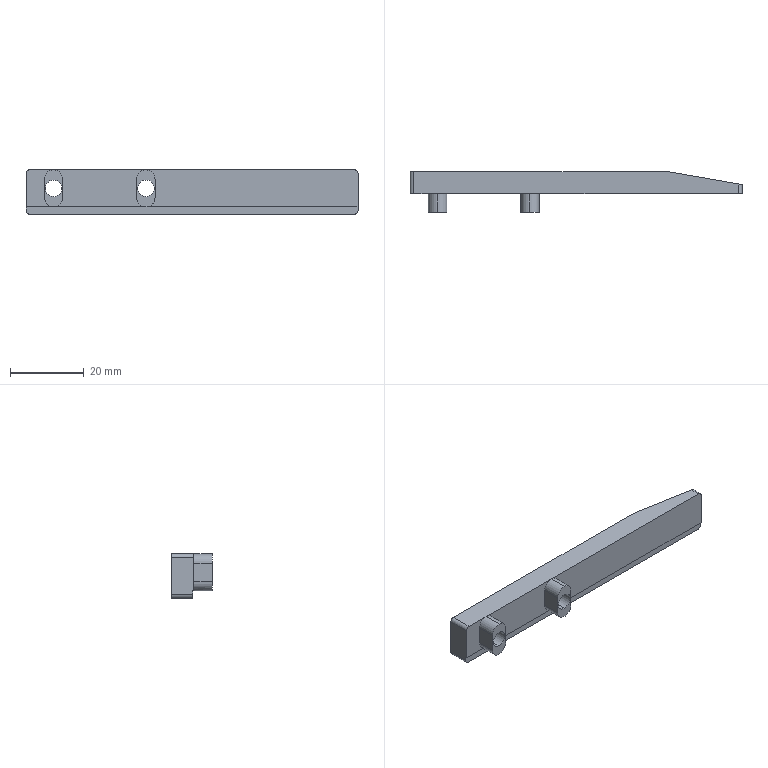Part | STEP file | 10000020606swp000-1 | 1 solid | 37 faces | box 90 x 11 x 12 mm | volume 5783 mm3 | plane 19 | cylinder 18 | commonest cylinder face diameters 5 x6 2 x4 4.5 x4 8 x4
STEP:
#1=CARTESIAN_POINT('',(7.5,1.4,-3.));
#2=VERTEX_POINT('',#1);
#3=CARTESIAN_POINT('',(7.5,1.4,5.));
#4=VERTEX_POINT('',#3);
#5=CARTESIAN_POINT('',(7.5,1.4,1.));
#6=DIRECTION('',(0.,1.,0.));
#7=DIRECTION('',(0.,0.,1.));
#8=AXIS2_PLACEMENT_3D('',#5,#6,#7);
#9=CIRCLE('',#8,4.);
#10=EDGE_CURVE('',#2,#4,#9,.T.);
#11=ORIENTED_EDGE('',*,*,#10,.F.);
#12=CARTESIAN_POINT('',(7.5,6.,-3.));
#13=VERTEX_POINT('',#12);
#14=CARTESIAN_POINT('',(7.5,6.,-3.));
#15=DIRECTION('',(0.,1.,0.));
#16=VECTOR('',#15,1000.);
#17=LINE('',#14,#16);
#18=EDGE_CURVE('',#2,#13,#17,.T.);
#19=ORIENTED_EDGE('',*,*,#18,.T.);
#20=CARTESIAN_POINT('',(7.5,6.,5.));
#21=VERTEX_POINT('',#20);
#22=CARTESIAN_POINT('',(7.5,6.,1.));
#23=DIRECTION('',(0.,1.,0.));
#24=DIRECTION('',(0.,0.,1.));
#25=AXIS2_PLACEMENT_3D('',#22,#23,#24);
#26=CIRCLE('',#25,4.);
#27=EDGE_CURVE('',#13,#21,#26,.T.);
#28=ORIENTED_EDGE('',*,*,#27,.T.);
#29=CARTESIAN_POINT('',(7.5,6.,5.));
#30=DIRECTION('',(0.,1.,0.));
#31=VECTOR('',#30,1000.);
#32=LINE('',#29,#31);
#33=EDGE_CURVE('',#4,#21,#32,.T.);
#34=ORIENTED_EDGE('',*,*,#33,.F.);
#35=EDGE_LOOP('',(#11,#19,#28,#34));
#36=FACE_OUTER_BOUND('',#35,.T.);
#37=CARTESIAN_POINT('',(7.5,6.,1.));
#38=DIRECTION('',(0.,1.,0.));
#39=DIRECTION('',(0.,0.,1.));
#40=AXIS2_PLACEMENT_3D('',#37,#38,#39);
#41=CYLINDRICAL_SURFACE('',#40,4.);
#42=ADVANCED_FACE('',(#36),#41,.F.);
#43=CARTESIAN_POINT('',(7.5,-5.,3.25));
#44=VERTEX_POINT('',#43);
#45=CARTESIAN_POINT('',(7.5,-5.,-1.25));
#46=VERTEX_POINT('',#45);
#47=CARTESIAN_POINT('',(7.5,-5.,1.));
#48=DIRECTION('',(0.,-1.,0.));
#49=DIRECTION('',(0.,0.,-1.));
#50=AXIS2_PLACEMENT_3D('',#47,#48,#49);
#51=CIRCLE('',#50,2.25);
#52=EDGE_CURVE('',#44,#46,#51,.T.);
#53=ORIENTED_EDGE('',*,*,#52,.T.);
#54=CARTESIAN_POINT('',(7.5,1.4,-1.25));
#55=VERTEX_POINT('',#54);
#56=CARTESIAN_POINT('',(7.5,6.,-1.25));
#57=DIRECTION('',(0.,1.,0.));
#58=VECTOR('',#57,1000.);
#59=LINE('',#56,#58);
#60=EDGE_CURVE('',#46,#55,#59,.T.);
#61=ORIENTED_EDGE('',*,*,#60,.T.);
#62=CARTESIAN_POINT('',(7.5,1.4,3.25));
#63=VERTEX_POINT('',#62);
#64=CARTESIAN_POINT('',(7.5,1.4,1.));
#65=DIRECTION('',(0.,1.,0.));
#66=DIRECTION('',(0.,0.,1.));
#67=AXIS2_PLACEMENT_3D('',#64,#65,#66);
#68=CIRCLE('',#67,2.25);
#69=EDGE_CURVE('',#55,#63,#68,.T.);
#70=ORIENTED_EDGE('',*,*,#69,.T.);
#71=CARTESIAN_POINT('',(7.5,6.,3.25));
#72=DIRECTION('',(0.,1.,0.));
#73=VECTOR('',#72,1000.);
#74=LINE('',#71,#73);
#75=EDGE_CURVE('',#44,#63,#74,.T.);
#76=ORIENTED_EDGE('',*,*,#75,.F.);
#77=EDGE_LOOP('',(#53,#61,#70,#76));
#78=FACE_OUTER_BOUND('',#77,.T.);
#79=CARTESIAN_POINT('',(7.5,6.,1.));
#80=DIRECTION('',(0.,1.,0.));
#81=DIRECTION('',(0.,0.,1.));
#82=AXIS2_PLACEMENT_3D('',#79,#80,#81);
#83=CYLINDRICAL_SURFACE('',#82,2.25);
#84=ADVANCED_FACE('',(#78),#83,.F.);
#85=CARTESIAN_POINT('',(32.5,1.4,-3.));
#86=VERTEX_POINT('',#85);
#87=CARTESIAN_POINT('',(32.5,1.4,5.));
#88=VERTEX_POINT('',#87);
#89=CARTESIAN_POINT('',(32.5,1.4,1.));
#90=DIRECTION('',(0.,1.,0.));
#91=DIRECTION('',(0.,0.,1.));
#92=AXIS2_PLACEMENT_3D('',#89,#90,#91);
#93=CIRCLE('',#92,4.);
#94=EDGE_CURVE('',#86,#88,#93,.T.);
#95=ORIENTED_EDGE('',*,*,#94,.F.);
#96=CARTESIAN_POINT('',(32.5,6.,-3.));
#97=VERTEX_POINT('',#96);
#98=CARTESIAN_POINT('',(32.5,6.,-3.));
#99=DIRECTION('',(0.,1.,0.));
#100=VECTOR('',#99,1000.);
#101=LINE('',#98,#100);
#102=EDGE_CURVE('',#86,#97,#101,.T.);
#103=ORIENTED_EDGE('',*,*,#102,.T.);
#104=CARTESIAN_POINT('',(32.5,6.,5.));
#105=VERTEX_POINT('',#104);
#106=CARTESIAN_POINT('',(32.5,6.,1.));
#107=DIRECTION('',(0.,1.,0.));
#108=DIRECTION('',(0.,0.,1.));
#109=AXIS2_PLACEMENT_3D('',#106,#107,#108);
#110=CIRCLE('',#109,4.);
#111=EDGE_CURVE('',#97,#105,#110,.T.);
#112=ORIENTED_EDGE('',*,*,#111,.T.);
#113=CARTESIAN_POINT('',(32.5,6.,5.));
#114=DIRECTION('',(0.,1.,0.));
#115=VECTOR('',#114,1000.);
#116=LINE('',#113,#115);
#117=EDGE_CURVE('',#88,#105,#116,.T.);
#118=ORIENTED_EDGE('',*,*,#117,.F.);
#119=EDGE_LOOP('',(#95,#103,#112,#118));
#120=FACE_OUTER_BOUND('',#119,.T.);
#121=CARTESIAN_POINT('',(32.5,6.,1.));
#122=DIRECTION('',(0.,1.,0.));
#123=DIRECTION('',(0.,0.,1.));
#124=AXIS2_PLACEMENT_3D('',#121,#122,#123);
#125=CYLINDRICAL_SURFACE('',#124,4.);
#126=ADVANCED_FACE('',(#120),#125,.F.);
#127=CARTESIAN_POINT('',(32.5,-5.,3.25));
#128=VERTEX_POINT('',#127);
#129=CARTESIAN_POINT('',(32.5,-5.,-1.25));
#130=VERTEX_POINT('',#129);
#131=CARTESIAN_POINT('',(32.5,-5.,1.));
#132=DIRECTION('',(0.,-1.,0.));
#133=DIRECTION('',(0.,0.,-1.));
#134=AXIS2_PLACEMENT_3D('',#131,#132,#133);
#135=CIRCLE('',#134,2.25);
#136=EDGE_CURVE('',#128,#130,#135,.T.);
#137=ORIENTED_EDGE('',*,*,#136,.T.);
#138=CARTESIAN_POINT('',(32.5,1.4,-1.25));
#139=VERTEX_POINT('',#138);
#140=CARTESIAN_POINT('',(32.5,6.,-1.25));
#141=DIRECTION('',(0.,1.,0.));
#142=VECTOR('',#141,1000.);
#143=LINE('',#140,#142);
#144=EDGE_CURVE('',#130,#139,#143,.T.);
#145=ORIENTED_EDGE('',*,*,#144,.T.);
#146=CARTESIAN_POINT('',(32.5,1.4,3.25));
#147=VERTEX_POINT('',#146);
#148=CARTESIAN_POINT('',(32.5,1.4,1.));
#149=DIRECTION('',(0.,1.,0.));
#150=DIRECTION('',(0.,0.,1.));
#151=AXIS2_PLACEMENT_3D('',#148,#149,#150);
#152=CIRCLE('',#151,2.25);
#153=EDGE_CURVE('',#139,#147,#152,.T.);
#154=ORIENTED_EDGE('',*,*,#153,.T.);
#155=CARTESIAN_POINT('',(32.5,6.,3.25));
#156=DIRECTION('',(0.,1.,0.));
#157=VECTOR('',#156,1000.);
#158=LINE('',#155,#157);
#159=EDGE_CURVE('',#128,#147,#158,.T.);
#160=ORIENTED_EDGE('',*,*,#159,.F.);
#161=EDGE_LOOP('',(#137,#145,#154,#160));
#162=FACE_OUTER_BOUND('',#161,.T.);
#163=CARTESIAN_POINT('',(32.5,6.,1.));
#164=DIRECTION('',(0.,1.,0.));
#165=DIRECTION('',(0.,0.,1.));
#166=AXIS2_PLACEMENT_3D('',#163,#164,#165);
#167=CYLINDRICAL_SURFACE('',#166,2.25);
#168=ADVANCED_FACE('',(#162),#167,.F.);
#169=CARTESIAN_POINT('',(32.5,-5.,6.));
#170=VERTEX_POINT('',#169);
#171=CARTESIAN_POINT('',(30.,-5.,3.5));
#172=VERTEX_POINT('',#171);
#173=CARTESIAN_POINT('',(32.5,-5.,3.5));
#174=DIRECTION('',(0.,-1.,0.));
#175=DIRECTION('',(0.,0.,-1.));
#176=AXIS2_PLACEMENT_3D('',#173,#174,#175);
#177=CIRCLE('',#176,2.5);
#178=EDGE_CURVE('',#170,#172,#177,.T.);
#179=ORIENTED_EDGE('',*,*,#178,.F.);
#180=CARTESIAN_POINT('',(32.5,0.,6.));
#181=VERTEX_POINT('',#180);
#182=CARTESIAN_POINT('',(32.5,-5.,6.));
#183=DIRECTION('',(0.,1.,0.));
#184=VECTOR('',#183,1000.);
#185=LINE('',#182,#184);
#186=EDGE_CURVE('',#170,#181,#185,.T.);
#187=ORIENTED_EDGE('',*,*,#186,.T.);
#188=CARTESIAN_POINT('',(30.,0.,3.5));
#189=VERTEX_POINT('',#188);
#190=CARTESIAN_POINT('',(32.5,0.,3.5));
#191=DIRECTION('',(0.,-1.,0.));
#192=DIRECTION('',(0.,0.,-1.));
#193=AXIS2_PLACEMENT_3D('',#190,#191,#192);
#194=CIRCLE('',#193,2.5);
#195=EDGE_CURVE('',#181,#189,#194,.T.);
#196=ORIENTED_EDGE('',*,*,#195,.T.);
#197=CARTESIAN_POINT('',(30.,-5.,3.5));
#198=DIRECTION('',(0.,1.,0.));
#199=VECTOR('',#198,1000.);
#200=LINE('',#197,#199);
#201=EDGE_CURVE('',#172,#189,#200,.T.);
#202=ORIENTED_EDGE('',*,*,#201,.F.);
#203=EDGE_LOOP('',(#179,#187,#196,#202));
#204=FACE_OUTER_BOUND('',#203,.T.);
#205=CARTESIAN_POINT('',(32.5,-5.,3.5));
#206=DIRECTION('',(0.,1.,0.));
#207=DIRECTION('',(0.,0.,1.));
#208=AXIS2_PLACEMENT_3D('',#205,#206,#207);
#209=CYLINDRICAL_SURFACE('',#208,2.5);
#210=ADVANCED_FACE('',(#204),#209,.T.);
#211=CARTESIAN_POINT('',(7.5,-5.,6.));
#212=VERTEX_POINT('',#211);
#213=CARTESIAN_POINT('',(5.,-5.,3.5));
#214=VERTEX_POINT('',#213);
#215=CARTESIAN_POINT('',(7.5,-5.,3.5));
#216=DIRECTION('',(0.,-1.,0.));
#217=DIRECTION('',(0.,0.,-1.));
#218=AXIS2_PLACEMENT_3D('',#215,#216,#217);
#219=CIRCLE('',#218,2.5);
#220=EDGE_CURVE('',#212,#214,#219,.T.);
#221=ORIENTED_EDGE('',*,*,#220,.F.);
#222=CARTESIAN_POINT('',(7.5,0.,6.));
#223=VERTEX_POINT('',#222);
#224=CARTESIAN_POINT('',(7.5,-5.,6.));
#225=DIRECTION('',(0.,1.,0.));
#226=VECTOR('',#225,1000.);
#227=LINE('',#224,#226);
#228=EDGE_CURVE('',#212,#223,#227,.T.);
#229=ORIENTED_EDGE('',*,*,#228,.T.);
#230=CARTESIAN_POINT('',(5.,0.,3.5));
#231=VERTEX_POINT('',#230);
#232=CARTESIAN_POINT('',(7.5,0.,3.5));
#233=DIRECTION('',(0.,-1.,0.));
#234=DIRECTION('',(0.,0.,-1.));
#235=AXIS2_PLACEMENT_3D('',#232,#233,#234);
#236=CIRCLE('',#235,2.5);
#237=EDGE_CURVE('',#223,#231,#236,.T.);
#238=ORIENTED_EDGE('',*,*,#237,.T.);
#239=CARTESIAN_POINT('',(5.,-5.,3.5));
#240=DIRECTION('',(0.,1.,0.));
#241=VECTOR('',#240,1000.);
#242=LINE('',#239,#241);
#243=EDGE_CURVE('',#214,#231,#242,.T.);
#244=ORIENTED_EDGE('',*,*,#243,.F.);
#245=EDGE_LOOP('',(#221,#229,#238,#244));
#246=FACE_OUTER_BOUND('',#245,.T.);
#247=CARTESIAN_POINT('',(7.5,-5.,3.5));
#248=DIRECTION('',(0.,1.,0.));
#249=DIRECTION('',(0.,0.,1.));
#250=AXIS2_PLACEMENT_3D('',#247,#248,#249);
#251=CYLINDRICAL_SURFACE('',#250,2.5);
#252=ADVANCED_FACE('',(#246),#251,.T.);
#253=CARTESIAN_POINT('',(90.,0.,5.));
#254=VERTEX_POINT('',#253);
#255=CARTESIAN_POINT('',(90.,0.,-4.));
#256=VERTEX_POINT('',#255);
#257=CARTESIAN_POINT('',(90.,0.,6.));
#258=DIRECTION('',(0.,0.,-1.));
#259=VECTOR('',#258,1000.);
#260=LINE('',#257,#259);
#261=EDGE_CURVE('',#254,#256,#260,.T.);
#262=ORIENTED_EDGE('',*,*,#261,.F.);
#263=CARTESIAN_POINT('',(89.,0.,6.));
#264=VERTEX_POINT('',#263);
#265=CARTESIAN_POINT('',(89.,0.,5.));
#266=DIRECTION('',(0.,-1.,0.));
#267=DIRECTION('',(0.,0.,1.));
#268=AXIS2_PLACEMENT_3D('',#265,#266,#267);
#269=CIRCLE('',#268,1.);
#270=EDGE_CURVE('',#254,#264,#269,.T.);
#271=ORIENTED_EDGE('',*,*,#270,.T.);
#272=CARTESIAN_POINT('',(0.,0.,6.));
#273=DIRECTION('',(1.,0.,0.));
#274=VECTOR('',#273,1000.);
#275=LINE('',#272,#274);
#276=EDGE_CURVE('',#181,#264,#275,.T.);
#277=ORIENTED_EDGE('',*,*,#276,.F.);
#278=CARTESIAN_POINT('',(35.,0.,3.5));
#279=VERTEX_POINT('',#278);
#280=CARTESIAN_POINT('',(32.5,0.,3.5));
#281=DIRECTION('',(0.,-1.,0.));
#282=DIRECTION('',(0.,0.,-1.));
#283=AXIS2_PLACEMENT_3D('',#280,#281,#282);
#284=CIRCLE('',#283,2.5);
#285=EDGE_CURVE('',#279,#181,#284,.T.);
#286=ORIENTED_EDGE('',*,*,#285,.F.);
#287=CARTESIAN_POINT('',(35.,0.,-1.5));
#288=VERTEX_POINT('',#287);
#289=CARTESIAN_POINT('',(35.,0.,3.5));
#290=DIRECTION('',(0.,0.,1.));
#291=VECTOR('',#290,1000.);
#292=LINE('',#289,#291);
#293=EDGE_CURVE('',#288,#279,#292,.T.);
#294=ORIENTED_EDGE('',*,*,#293,.F.);
#295=CARTESIAN_POINT('',(32.5,0.,-4.));
#296=VERTEX_POINT('',#295);
#297=CARTESIAN_POINT('',(32.5,0.,-1.5));
#298=DIRECTION('',(0.,-1.,0.));
#299=DIRECTION('',(0.,0.,-1.));
#300=AXIS2_PLACEMENT_3D('',#297,#298,#299);
#301=CIRCLE('',#300,2.5);
#302=EDGE_CURVE('',#296,#288,#301,.T.);
#303=ORIENTED_EDGE('',*,*,#302,.F.);
#304=CARTESIAN_POINT('',(90.,0.,-4.));
#305=DIRECTION('',(1.,0.,0.));
#306=VECTOR('',#305,1000.);
#307=LINE('',#304,#306);
#308=EDGE_CURVE('',#296,#256,#307,.T.);
#309=ORIENTED_EDGE('',*,*,#308,.T.);
#310=EDGE_LOOP('',(#262,#271,#277,#286,#294,#303,#309));
#311=FACE_OUTER_BOUND('',#310,.T.);
#312=CARTESIAN_POINT('',(0.,0.,6.));
#313=DIRECTION('',(0.,1.,0.));
#314=DIRECTION('',(0.,0.,1.));
#315=AXIS2_PLACEMENT_3D('',#312,#313,#314);
#316=PLANE('',#315);
#317=ADVANCED_FACE('',(#311),#316,.F.);
#318=ORIENTED_EDGE('',*,*,#195,.F.);
#319=CARTESIAN_POINT('',(0.,0.,6.));
#320=DIRECTION('',(1.,0.,0.));
#321=VECTOR('',#320,1000.);
#322=LINE('',#319,#321);
#323=EDGE_CURVE('',#223,#181,#322,.T.);
#324=ORIENTED_EDGE('',*,*,#323,.F.);
#325=CARTESIAN_POINT('',(10.,0.,3.5));
#326=VERTEX_POINT('',#325);
#327=CARTESIAN_POINT('',(7.5,0.,3.5));
#328=DIRECTION('',(0.,-1.,0.));
#329=DIRECTION('',(0.,0.,-1.));
#330=AXIS2_PLACEMENT_3D('',#327,#328,#329);
#331=CIRCLE('',#330,2.5);
#332=EDGE_CURVE('',#326,#223,#331,.T.);
#333=ORIENTED_EDGE('',*,*,#332,.F.);
#334=CARTESIAN_POINT('',(10.,0.,-1.5));
#335=VERTEX_POINT('',#334);
#336=CARTESIAN_POINT('',(10.,0.,3.5));
#337=DIRECTION('',(0.,0.,1.));
#338=VECTOR('',#337,1000.);
#339=LINE('',#336,#338);
#340=EDGE_CURVE('',#335,#326,#339,.T.);
#341=ORIENTED_EDGE('',*,*,#340,.F.);
#342=CARTESIAN_POINT('',(7.5,0.,-4.));
#343=VERTEX_POINT('',#342);
#344=CARTESIAN_POINT('',(7.5,0.,-1.5));
#345=DIRECTION('',(0.,-1.,0.));
#346=DIRECTION('',(0.,0.,-1.));
#347=AXIS2_PLACEMENT_3D('',#344,#345,#346);
#348=CIRCLE('',#347,2.5);
#349=EDGE_CURVE('',#343,#335,#348,.T.);
#350=ORIENTED_EDGE('',*,*,#349,.F.);
#351=CARTESIAN_POINT('',(90.,0.,-4.));
#352=DIRECTION('',(1.,0.,0.));
#353=VECTOR('',#352,1000.);
#354=LINE('',#351,#353);
#355=EDGE_CURVE('',#343,#296,#354,.T.);
#356=ORIENTED_EDGE('',*,*,#355,.T.);
#357=CARTESIAN_POINT('',(30.,0.,-1.5));
#358=VERTEX_POINT('',#357);
#359=CARTESIAN_POINT('',(32.5,0.,-1.5));
#360=DIRECTION('',(0.,-1.,0.));
#361=DIRECTION('',(0.,0.,-1.));
#362=AXIS2_PLACEMENT_3D('',#359,#360,#361);
#363=CIRCLE('',#362,2.5);
#364=EDGE_CURVE('',#358,#296,#363,.T.);
#365=ORIENTED_EDGE('',*,*,#364,.F.);
#366=CARTESIAN_POINT('',(30.,0.,3.5));
#367=DIRECTION('',(0.,0.,-1.));
#368=VECTOR('',#367,1000.);
#369=LINE('',#366,#368);
#370=EDGE_CURVE('',#189,#358,#369,.T.);
#371=ORIENTED_EDGE('',*,*,#370,.F.);
#372=EDGE_LOOP('',(#318,#324,#333,#341,#350,#356,#365,#371));
#373=FACE_OUTER_BOUND('',#372,.T.);
#374=CARTESIAN_POINT('',(0.,0.,6.));
#375=DIRECTION('',(0.,1.,0.));
#376=DIRECTION('',(0.,0.,1.));
#377=AXIS2_PLACEMENT_3D('',#374,#375,#376);
#378=PLANE('',#377);
#379=ADVANCED_FACE('',(#373),#378,.F.);
#380=CARTESIAN_POINT('',(1.,0.,6.));
#381=VERTEX_POINT('',#380);
#382=CARTESIAN_POINT('',(0.,0.,6.));
#383=DIRECTION('',(1.,0.,0.));
#384=VECTOR('',#383,1000.);
#385=LINE('',#382,#384);
#386=EDGE_CURVE('',#381,#223,#385,.T.);
#387=ORIENTED_EDGE('',*,*,#386,.F.);
#388=CARTESIAN_POINT('',(0.,0.,5.));
#389=VERTEX_POINT('',#388);
#390=CARTESIAN_POINT('',(1.,0.,5.));
#391=DIRECTION('',(0.,-1.,0.));
#392=DIRECTION('',(0.,0.,1.));
#393=AXIS2_PLACEMENT_3D('',#390,#391,#392);
#394=CIRCLE('',#393,1.);
#395=EDGE_CURVE('',#381,#389,#394,.T.);
#396=ORIENTED_EDGE('',*,*,#395,.T.);
#397=CARTESIAN_POINT('',(0.,0.,-4.));
#398=VERTEX_POINT('',#397);
#399=CARTESIAN_POINT('',(0.,0.,6.));
#400=DIRECTION('',(0.,0.,-1.));
#401=VECTOR('',#400,1000.);
#402=LINE('',#399,#401);
#403=EDGE_CURVE('',#389,#398,#402,.T.);
#404=ORIENTED_EDGE('',*,*,#403,.T.);
#405=CARTESIAN_POINT('',(90.,0.,-4.));
#406=DIRECTION('',(1.,0.,0.));
#407=VECTOR('',#406,1000.);
#408=LINE('',#405,#407);
#409=EDGE_CURVE('',#398,#343,#408,.T.);
#410=ORIENTED_EDGE('',*,*,#409,.T.);
#411=CARTESIAN_POINT('',(5.,0.,-1.5));
#412=VERTEX_POINT('',#411);
#413=CARTESIAN_POINT('',(7.5,0.,-1.5));
#414=DIRECTION('',(0.,-1.,0.));
#415=DIRECTION('',(0.,0.,-1.));
#416=AXIS2_PLACEMENT_3D('',#413,#414,#415);
#417=CIRCLE('',#416,2.5);
#418=EDGE_CURVE('',#412,#343,#417,.T.);
#419=ORIENTED_EDGE('',*,*,#418,.F.);
#420=CARTESIAN_POINT('',(5.,0.,3.5));
#421=DIRECTION('',(0.,0.,-1.));
#422=VECTOR('',#421,1000.);
#423=LINE('',#420,#422);
#424=EDGE_CURVE('',#231,#412,#423,.T.);
#425=ORIENTED_EDGE('',*,*,#424,.F.);
#426=ORIENTED_EDGE('',*,*,#237,.F.);
#427=EDGE_LOOP('',(#387,#396,#404,#410,#419,#425,#426));
#428=FACE_OUTER_BOUND('',#427,.T.);
#429=CARTESIAN_POINT('',(0.,0.,6.));
#430=DIRECTION('',(0.,1.,0.));
#431=DIRECTION('',(0.,0.,1.));
#432=AXIS2_PLACEMENT_3D('',#429,#430,#431);
#433=PLANE('',#432);
#434=ADVANCED_FACE('',(#428),#433,.F.);
#435=CARTESIAN_POINT('',(0.,6.,5.));
#436=VERTEX_POINT('',#435);
#437=CARTESIAN_POINT('',(0.,6.,-5.));
#438=VERTEX_POINT('',#437);
#439=CARTESIAN_POINT('',(0.,6.,6.));
#440=DIRECTION('',(0.,0.,-1.));
#441=VECTOR('',#440,1000.);
#442=LINE('',#439,#441);
#443=EDGE_CURVE('',#436,#438,#442,.T.);
#444=ORIENTED_EDGE('',*,*,#443,.T.);
#445=CARTESIAN_POINT('',(0.,0.3,-5.));
#446=VERTEX_POINT('',#445);
#447=CARTESIAN_POINT('',(0.,0.3,-5.));
#448=DIRECTION('',(0.,-1.,0.));
#449=VECTOR('',#448,1000.);
#450=LINE('',#447,#449);
#451=EDGE_CURVE('',#438,#446,#450,.T.);
#452=ORIENTED_EDGE('',*,*,#451,.T.);
#453=CARTESIAN_POINT('',(0.,0.3,-4.));
#454=VERTEX_POINT('',#453);
#455=CARTESIAN_POINT('',(0.,0.3,-4.));
#456=DIRECTION('',(0.,0.,-1.));
#457=VECTOR('',#456,1000.);
#458=LINE('',#455,#457);
#459=EDGE_CURVE('',#454,#446,#458,.T.);
#460=ORIENTED_EDGE('',*,*,#459,.F.);
#461=CARTESIAN_POINT('',(0.,0.,-4.));
#462=DIRECTION('',(0.,-1.,0.));
#463=VECTOR('',#462,1000.);
#464=LINE('',#461,#463);
#465=EDGE_CURVE('',#454,#398,#464,.T.);
#466=ORIENTED_EDGE('',*,*,#465,.T.);
#467=ORIENTED_EDGE('',*,*,#403,.F.);
#468=CARTESIAN_POINT('',(0.,0.,5.));
#469=DIRECTION('',(0.,1.,0.));
#470=VECTOR('',#469,1000.);
#471=LINE('',#468,#470);
#472=EDGE_CURVE('',#389,#436,#471,.T.);
#473=ORIENTED_EDGE('',*,*,#472,.T.);
#474=EDGE_LOOP('',(#444,#452,#460,#466,#467,#473));
#475=FACE_OUTER_BOUND('',#474,.T.);
#476=CARTESIAN_POINT('',(0.,0.,6.));
#477=DIRECTION('',(1.,0.,0.));
#478=DIRECTION('',(0.,0.,-1.));
#479=AXIS2_PLACEMENT_3D('',#476,#477,#478);
#480=PLANE('',#479);
#481=ADVANCED_FACE('',(#475),#480,.F.);
#482=CARTESIAN_POINT('',(90.,0.3,-4.));
#483=VERTEX_POINT('',#482);
#484=CARTESIAN_POINT('',(90.,0.3,-5.));
#485=VERTEX_POINT('',#484);
#486=CARTESIAN_POINT('',(90.,0.3,-4.));
#487=DIRECTION('',(0.,0.,-1.));
#488=VECTOR('',#487,1000.);
#489=LINE('',#486,#488);
#490=EDGE_CURVE('',#483,#485,#489,.T.);
#491=ORIENTED_EDGE('',*,*,#490,.T.);
#492=CARTESIAN_POINT('',(90.,2.5,-5.));
#493=VERTEX_POINT('',#492);
#494=CARTESIAN_POINT('',(90.,2.5,-5.));
#495=DIRECTION('',(0.,1.,0.));
#496=VECTOR('',#495,1000.);
#497=LINE('',#494,#496);
#498=EDGE_CURVE('',#485,#493,#497,.T.);
#499=ORIENTED_EDGE('',*,*,#498,.T.);
#500=CARTESIAN_POINT('',(90.,2.5,5.));
#501=VERTEX_POINT('',#500);
#502=CARTESIAN_POINT('',(90.,2.5,6.));
#503=DIRECTION('',(0.,0.,-1.));
#504=VECTOR('',#503,1000.);
#505=LINE('',#502,#504);
#506=EDGE_CURVE('',#501,#493,#505,.T.);
#507=ORIENTED_EDGE('',*,*,#506,.F.);
#508=CARTESIAN_POINT('',(90.,0.,5.));
#509=DIRECTION('',(0.,-1.,0.));
#510=VECTOR('',#509,1000.);
#511=LINE('',#508,#510);
#512=EDGE_CURVE('',#501,#254,#511,.T.);
#513=ORIENTED_EDGE('',*,*,#512,.T.);
#514=ORIENTED_EDGE('',*,*,#261,.T.);
#515=CARTESIAN_POINT('',(90.,0.,-4.));
#516=DIRECTION('',(0.,1.,0.));
#517=VECTOR('',#516,1000.);
#518=LINE('',#515,#517);
#519=EDGE_CURVE('',#256,#483,#518,.T.);
#520=ORIENTED_EDGE('',*,*,#519,.T.);
#521=EDGE_LOOP('',(#491,#499,#507,#513,#514,#520));
#522=FACE_OUTER_BOUND('',#521,.T.);
#523=CARTESIAN_POINT('',(90.,0.,6.));
#524=DIRECTION('',(-1.,0.,0.));
#525=DIRECTION('',(0.,0.,1.));
#526=AXIS2_PLACEMENT_3D('',#523,#524,#525);
#527=PLANE('',#526);
#528=ADVANCED_FACE('',(#522),#527,.F.);
#529=CARTESIAN_POINT('',(89.,0.3,-6.));
#530=VERTEX_POINT('',#529);
#531=CARTESIAN_POINT('',(1.,0.3,-6.));
#532=VERTEX_POINT('',#531);
#533=CARTESIAN_POINT('',(90.,0.3,-6.));
#534=DIRECTION('',(-1.,0.,0.));
#535=VECTOR('',#534,1000.);
#536=LINE('',#533,#535);
#537=EDGE_CURVE('',#530,#532,#536,.T.);
#538=ORIENTED_EDGE('',*,*,#537,.T.);
#539=CARTESIAN_POINT('',(1.,6.,-6.));
#540=VERTEX_POINT('',#539);
#541=CARTESIAN_POINT('',(1.,6.,-6.));
#542=DIRECTION('',(0.,1.,0.));
#543=VECTOR('',#542,1000.);
#544=LINE('',#541,#543);
#545=EDGE_CURVE('',#532,#540,#544,.T.);
#546=ORIENTED_EDGE('',*,*,#545,.T.);
#547=CARTESIAN_POINT('',(70.,6.,-6.));
#548=VERTEX_POINT('',#547);
#549=CARTESIAN_POINT('',(0.,6.,-6.));
#550=DIRECTION('',(-1.,0.,0.));
#551=VECTOR('',#550,1000.);
#552=LINE('',#549,#551);
#553=EDGE_CURVE('',#548,#540,#552,.T.);
#554=ORIENTED_EDGE('',*,*,#553,.F.);
#555=CARTESIAN_POINT('',(89.,2.675,-6.));
#556=VERTEX_POINT('',#555);
#557=CARTESIAN_POINT('',(90.,2.5,-6.));
#558=DIRECTION('',(-0.985,0.1724,0.));
#559=VECTOR('',#558,1000.);
#560=LINE('',#557,#559);
#561=EDGE_CURVE('',#556,#548,#560,.T.);
#562=ORIENTED_EDGE('',*,*,#561,.F.);
#563=CARTESIAN_POINT('',(89.,0.3,-6.));
#564=DIRECTION('',(0.,-1.,0.));
#565=VECTOR('',#564,1000.);
#566=LINE('',#563,#565);
#567=EDGE_CURVE('',#556,#530,#566,.T.);
#568=ORIENTED_EDGE('',*,*,#567,.T.);
#569=EDGE_LOOP('',(#538,#546,#554,#562,#568));
#570=FACE_OUTER_BOUND('',#569,.T.);
#571=CARTESIAN_POINT('',(0.,0.,-6.));
#572=DIRECTION('',(0.,0.,-1.));
#573=DIRECTION('',(-1.,0.,0.));
#574=AXIS2_PLACEMENT_3D('',#571,#572,#573);
#575=PLANE('',#574);
#576=ADVANCED_FACE('',(#570),#575,.T.);
#577=ORIENTED_EDGE('',*,*,#506,.T.);
#578=CARTESIAN_POINT('',(90.,2.5,-5.));
#579=CARTESIAN_POINT('',(90.,2.5,-5.586));
#580=CARTESIAN_POINT('',(89.586,2.572,-6.));
#581=CARTESIAN_POINT('',(89.,2.675,-6.));
#582=(BOUNDED_CURVE()B_SPLINE_CURVE(3,(#578,#579,#580,#581),.UNSPECIFIED.,.F.,.F.)B_SPLINE_CURVE_WITH_KNOTS((4,4),(0.,1.571),.UNSPECIFIED.)CURVE()GEOMETRIC_REPRESENTATION_ITEM()RATIONAL_B_SPLINE_CURVE((1.,0.8047,0.8047,1.))REPRESENTATION_ITEM(''));
#583=EDGE_CURVE('',#493,#556,#582,.T.);
#584=ORIENTED_EDGE('',*,*,#583,.T.);
#585=ORIENTED_EDGE('',*,*,#561,.T.);
#586=CARTESIAN_POINT('',(70.,6.,6.));
#587=VERTEX_POINT('',#586);
#588=CARTESIAN_POINT('',(70.,6.,6.));
#589=DIRECTION('',(0.,0.,-1.));
#590=VECTOR('',#589,1000.);
#591=LINE('',#588,#590);
#592=EDGE_CURVE('',#587,#548,#591,.T.);
#593=ORIENTED_EDGE('',*,*,#592,.F.);
#594=CARTESIAN_POINT('',(89.,2.675,6.));
#595=VERTEX_POINT('',#594);
#596=CARTESIAN_POINT('',(90.,2.5,6.));
#597=DIRECTION('',(-0.985,0.1724,0.));
#598=VECTOR('',#597,1000.);
#599=LINE('',#596,#598);
#600=EDGE_CURVE('',#595,#587,#599,.T.);
#601=ORIENTED_EDGE('',*,*,#600,.F.);
#602=CARTESIAN_POINT('',(89.,2.675,6.));
#603=CARTESIAN_POINT('',(89.586,2.572,6.));
#604=CARTESIAN_POINT('',(90.,2.5,5.586));
#605=CARTESIAN_POINT('',(90.,2.5,5.));
#606=(BOUNDED_CURVE()B_SPLINE_CURVE(3,(#602,#603,#604,#605),.UNSPECIFIED.,.F.,.F.)B_SPLINE_CURVE_WITH_KNOTS((4,4),(1.571,3.142),.UNSPECIFIED.)CURVE()GEOMETRIC_REPRESENTATION_ITEM()RATIONAL_B_SPLINE_CURVE((1.,0.8047,0.8047,1.))REPRESENTATION_ITEM(''));
#607=EDGE_CURVE('',#595,#501,#606,.T.);
#608=ORIENTED_EDGE('',*,*,#607,.T.);
#609=EDGE_LOOP('',(#577,#584,#585,#593,#601,#608));
#610=FACE_OUTER_BOUND('',#609,.T.);
#611=CARTESIAN_POINT('',(90.,2.5,6.));
#612=DIRECTION('',(-0.1724,-0.985,0.));
#613=DIRECTION('',(0.985,-0.1724,0.));
#614=AXIS2_PLACEMENT_3D('',#611,#612,#613);
#615=PLANE('',#614);
#616=ADVANCED_FACE('',(#610),#615,.F.);
#617=CARTESIAN_POINT('',(7.5,6.,1.));
#618=DIRECTION('',(0.,1.,0.));
#619=DIRECTION('',(0.,0.,1.));
#620=AXIS2_PLACEMENT_3D('',#617,#618,#619);
#621=CIRCLE('',#620,4.);
#622=EDGE_CURVE('',#21,#13,#621,.T.);
#623=ORIENTED_EDGE('',*,*,#622,.F.);
#624=ORIENTED_EDGE('',*,*,#27,.F.);
#625=EDGE_LOOP('',(#623,#624));
#626=FACE_BOUND('',#625,.T.);
#627=CARTESIAN_POINT('',(32.5,6.,1.));
#628=DIRECTION('',(0.,1.,0.));
#629=DIRECTION('',(0.,0.,1.));
#630=AXIS2_PLACEMENT_3D('',#627,#628,#629);
#631=CIRCLE('',#630,4.);
#632=EDGE_CURVE('',#105,#97,#631,.T.);
#633=ORIENTED_EDGE('',*,*,#632,.F.);
#634=ORIENTED_EDGE('',*,*,#111,.F.);
#635=EDGE_LOOP('',(#633,#634));
#636=FACE_BOUND('',#635,.T.);
#637=ORIENTED_EDGE('',*,*,#553,.T.);
#638=CARTESIAN_POINT('',(1.,6.,-5.));
#639=DIRECTION('',(0.,1.,0.));
#640=DIRECTION('',(0.,0.,-1.));
#641=AXIS2_PLACEMENT_3D('',#638,#639,#640);
#642=CIRCLE('',#641,1.);
#643=EDGE_CURVE('',#540,#438,#642,.T.);
#644=ORIENTED_EDGE('',*,*,#643,.T.);
#645=ORIENTED_EDGE('',*,*,#443,.F.);
#646=CARTESIAN_POINT('',(1.,6.,6.));
#647=VERTEX_POINT('',#646);
#648=CARTESIAN_POINT('',(1.,6.,5.));
#649=DIRECTION('',(0.,1.,0.));
#650=DIRECTION('',(0.,0.,-1.));
#651=AXIS2_PLACEMENT_3D('',#648,#649,#650);
#652=CIRCLE('',#651,1.);
#653=EDGE_CURVE('',#436,#647,#652,.T.);
#654=ORIENTED_EDGE('',*,*,#653,.T.);
#655=CARTESIAN_POINT('',(0.,6.,6.));
#656=DIRECTION('',(-1.,0.,0.));
#657=VECTOR('',#656,1000.);
#658=LINE('',#655,#657);
#659=EDGE_CURVE('',#587,#647,#658,.T.);
#660=ORIENTED_EDGE('',*,*,#659,.F.);
#661=ORIENTED_EDGE('',*,*,#592,.T.);
#662=EDGE_LOOP('',(#637,#644,#645,#654,#660,#661));
#663=FACE_OUTER_BOUND('',#662,.T.);
#664=CARTESIAN_POINT('',(0.,6.,6.));
#665=DIRECTION('',(0.,-1.,0.));
#666=DIRECTION('',(0.,0.,-1.));
#667=AXIS2_PLACEMENT_3D('',#664,#665,#666);
#668=PLANE('',#667);
#669=ADVANCED_FACE('',(#626,#636,#663),#668,.F.);
#670=ORIENTED_EDGE('',*,*,#659,.T.);
#671=CARTESIAN_POINT('',(1.,0.,6.));
#672=DIRECTION('',(0.,-1.,0.));
#673=VECTOR('',#672,1000.);
#674=LINE('',#671,#673);
#675=EDGE_CURVE('',#647,#381,#674,.T.);
#676=ORIENTED_EDGE('',*,*,#675,.T.);
#677=ORIENTED_EDGE('',*,*,#386,.T.);
#678=ORIENTED_EDGE('',*,*,#323,.T.);
#679=ORIENTED_EDGE('',*,*,#276,.T.);
#680=CARTESIAN_POINT('',(89.,0.,6.));
#681=DIRECTION('',(0.,1.,0.));
#682=VECTOR('',#681,1000.);
#683=LINE('',#680,#682);
#684=EDGE_CURVE('',#264,#595,#683,.T.);
#685=ORIENTED_EDGE('',*,*,#684,.T.);
#686=ORIENTED_EDGE('',*,*,#600,.T.);
#687=EDGE_LOOP('',(#670,#676,#677,#678,#679,#685,#686));
#688=FACE_OUTER_BOUND('',#687,.T.);
#689=CARTESIAN_POINT('',(0.,0.,6.));
#690=DIRECTION('',(0.,0.,-1.));
#691=DIRECTION('',(-1.,0.,0.));
#692=AXIS2_PLACEMENT_3D('',#689,#690,#691);
#693=PLANE('',#692);
#694=ADVANCED_FACE('',(#688),#693,.F.);
#695=ORIENTED_EDGE('',*,*,#459,.T.);
#696=CARTESIAN_POINT('',(1.,0.3,-5.));
#697=DIRECTION('',(0.,-1.,0.));
#698=DIRECTION('',(1.,0.,0.));
#699=AXIS2_PLACEMENT_3D('',#696,#697,#698);
#700=CIRCLE('',#699,1.);
#701=EDGE_CURVE('',#446,#532,#700,.T.);
#702=ORIENTED_EDGE('',*,*,#701,.T.);
#703=ORIENTED_EDGE('',*,*,#537,.F.);
#704=CARTESIAN_POINT('',(89.,0.3,-5.));
#705=DIRECTION('',(0.,-1.,0.));
#706=DIRECTION('',(1.,0.,0.));
#707=AXIS2_PLACEMENT_3D('',#704,#705,#706);
#708=CIRCLE('',#707,1.);
#709=EDGE_CURVE('',#530,#485,#708,.T.);
#710=ORIENTED_EDGE('',*,*,#709,.T.);
#711=ORIENTED_EDGE('',*,*,#490,.F.);
#712=CARTESIAN_POINT('',(90.,0.3,-4.));
#713=DIRECTION('',(-1.,0.,0.));
#714=VECTOR('',#713,1000.);
#715=LINE('',#712,#714);
#716=EDGE_CURVE('',#483,#454,#715,.T.);
#717=ORIENTED_EDGE('',*,*,#716,.T.);
#718=EDGE_LOOP('',(#695,#702,#703,#710,#711,#717));
#719=FACE_OUTER_BOUND('',#718,.T.);
#720=CARTESIAN_POINT('',(90.,0.3,-4.));
#721=DIRECTION('',(0.,-1.,0.));
#722=DIRECTION('',(1.,0.,0.));
#723=AXIS2_PLACEMENT_3D('',#720,#721,#722);
#724=PLANE('',#723);
#725=ADVANCED_FACE('',(#719),#724,.T.);
#726=ORIENTED_EDGE('',*,*,#519,.F.);
#727=ORIENTED_EDGE('',*,*,#308,.F.);
#728=ORIENTED_EDGE('',*,*,#355,.F.);
#729=ORIENTED_EDGE('',*,*,#409,.F.);
#730=ORIENTED_EDGE('',*,*,#465,.F.);
#731=ORIENTED_EDGE('',*,*,#716,.F.);
#732=EDGE_LOOP('',(#726,#727,#728,#729,#730,#731));
#733=FACE_OUTER_BOUND('',#732,.T.);
#734=CARTESIAN_POINT('',(0.,0.,-4.));
#735=DIRECTION('',(0.,0.,1.));
#736=DIRECTION('',(1.,0.,0.));
#737=AXIS2_PLACEMENT_3D('',#734,#735,#736);
#738=PLANE('',#737);
#739=ADVANCED_FACE('',(#733),#738,.F.);
#740=ORIENTED_EDGE('',*,*,#228,.F.);
#741=CARTESIAN_POINT('',(10.,-5.,3.5));
#742=VERTEX_POINT('',#741);
#743=CARTESIAN_POINT('',(7.5,-5.,3.5));
#744=DIRECTION('',(0.,-1.,0.));
#745=DIRECTION('',(0.,0.,-1.));
#746=AXIS2_PLACEMENT_3D('',#743,#744,#745);
#747=CIRCLE('',#746,2.5);
#748=EDGE_CURVE('',#742,#212,#747,.T.);
#749=ORIENTED_EDGE('',*,*,#748,.F.);
#750=CARTESIAN_POINT('',(10.,-5.,3.5));
#751=DIRECTION('',(0.,1.,0.));
#752=VECTOR('',#751,1000.);
#753=LINE('',#750,#752);
#754=EDGE_CURVE('',#742,#326,#753,.T.);
#755=ORIENTED_EDGE('',*,*,#754,.T.);
#756=ORIENTED_EDGE('',*,*,#332,.T.);
#757=EDGE_LOOP('',(#740,#749,#755,#756));
#758=FACE_OUTER_BOUND('',#757,.T.);
#759=CARTESIAN_POINT('',(7.5,-5.,3.5));
#760=DIRECTION('',(0.,1.,0.));
#761=DIRECTION('',(0.,0.,1.));
#762=AXIS2_PLACEMENT_3D('',#759,#760,#761);
#763=CYLINDRICAL_SURFACE('',#762,2.5);
#764=ADVANCED_FACE('',(#758),#763,.T.);
#765=ORIENTED_EDGE('',*,*,#424,.T.);
#766=CARTESIAN_POINT('',(5.,-5.,-1.5));
#767=VERTEX_POINT('',#766);
#768=CARTESIAN_POINT('',(5.,-5.,-1.5));
#769=DIRECTION('',(0.,1.,0.));
#770=VECTOR('',#769,1000.);
#771=LINE('',#768,#770);
#772=EDGE_CURVE('',#767,#412,#771,.T.);
#773=ORIENTED_EDGE('',*,*,#772,.F.);
#774=CARTESIAN_POINT('',(5.,-5.,3.5));
#775=DIRECTION('',(0.,0.,-1.));
#776=VECTOR('',#775,1000.);
#777=LINE('',#774,#776);
#778=EDGE_CURVE('',#214,#767,#777,.T.);
#779=ORIENTED_EDGE('',*,*,#778,.F.);
#780=ORIENTED_EDGE('',*,*,#243,.T.);
#781=EDGE_LOOP('',(#765,#773,#779,#780));
#782=FACE_OUTER_BOUND('',#781,.T.);
#783=CARTESIAN_POINT('',(5.,-5.,3.5));
#784=DIRECTION('',(1.,0.,0.));
#785=DIRECTION('',(0.,0.,-1.));
#786=AXIS2_PLACEMENT_3D('',#783,#784,#785);
#787=PLANE('',#786);
#788=ADVANCED_FACE('',(#782),#787,.F.);
#789=ORIENTED_EDGE('',*,*,#418,.T.);
#790=ORIENTED_EDGE('',*,*,#349,.T.);
#791=CARTESIAN_POINT('',(10.,-5.,-1.5));
#792=VERTEX_POINT('',#791);
#793=CARTESIAN_POINT('',(10.,-5.,-1.5));
#794=DIRECTION('',(0.,1.,0.));
#795=VECTOR('',#794,1000.);
#796=LINE('',#793,#795);
#797=EDGE_CURVE('',#792,#335,#796,.T.);
#798=ORIENTED_EDGE('',*,*,#797,.F.);
#799=CARTESIAN_POINT('',(7.5,-5.,-1.5));
#800=DIRECTION('',(0.,-1.,0.));
#801=DIRECTION('',(0.,0.,-1.));
#802=AXIS2_PLACEMENT_3D('',#799,#800,#801);
#803=CIRCLE('',#802,2.5);
#804=EDGE_CURVE('',#767,#792,#803,.T.);
#805=ORIENTED_EDGE('',*,*,#804,.F.);
#806=ORIENTED_EDGE('',*,*,#772,.T.);
#807=EDGE_LOOP('',(#789,#790,#798,#805,#806));
#808=FACE_OUTER_BOUND('',#807,.T.);
#809=CARTESIAN_POINT('',(7.5,-5.,-1.5));
#810=DIRECTION('',(0.,1.,0.));
#811=DIRECTION('',(0.,0.,1.));
#812=AXIS2_PLACEMENT_3D('',#809,#810,#811);
#813=CYLINDRICAL_SURFACE('',#812,2.5);
#814=ADVANCED_FACE('',(#808),#813,.T.);
#815=ORIENTED_EDGE('',*,*,#340,.T.);
#816=ORIENTED_EDGE('',*,*,#754,.F.);
#817=CARTESIAN_POINT('',(10.,-5.,3.5));
#818=DIRECTION('',(0.,0.,1.));
#819=VECTOR('',#818,1000.);
#820=LINE('',#817,#819);
#821=EDGE_CURVE('',#792,#742,#820,.T.);
#822=ORIENTED_EDGE('',*,*,#821,.F.);
#823=ORIENTED_EDGE('',*,*,#797,.T.);
#824=EDGE_LOOP('',(#815,#816,#822,#823));
#825=FACE_OUTER_BOUND('',#824,.T.);
#826=CARTESIAN_POINT('',(10.,-5.,3.5));
#827=DIRECTION('',(-1.,0.,0.));
#828=DIRECTION('',(0.,0.,1.));
#829=AXIS2_PLACEMENT_3D('',#826,#827,#828);
#830=PLANE('',#829);
#831=ADVANCED_FACE('',(#825),#830,.F.);
#832=ORIENTED_EDGE('',*,*,#52,.F.);
#833=CARTESIAN_POINT('',(7.5,-5.,1.));
#834=DIRECTION('',(0.,-1.,0.));
#835=DIRECTION('',(0.,0.,-1.));
#836=AXIS2_PLACEMENT_3D('',#833,#834,#835);
#837=CIRCLE('',#836,2.25);
#838=EDGE_CURVE('',#46,#44,#837,.T.);
#839=ORIENTED_EDGE('',*,*,#838,.F.);
#840=EDGE_LOOP('',(#832,#839));
#841=FACE_BOUND('',#840,.T.);
#842=ORIENTED_EDGE('',*,*,#748,.T.);
#843=ORIENTED_EDGE('',*,*,#220,.T.);
#844=ORIENTED_EDGE('',*,*,#778,.T.);
#845=ORIENTED_EDGE('',*,*,#804,.T.);
#846=ORIENTED_EDGE('',*,*,#821,.T.);
#847=EDGE_LOOP('',(#842,#843,#844,#845,#846));
#848=FACE_OUTER_BOUND('',#847,.T.);
#849=CARTESIAN_POINT('',(7.5,-5.,3.5));
#850=DIRECTION('',(0.,-1.,0.));
#851=DIRECTION('',(0.,0.,-1.));
#852=AXIS2_PLACEMENT_3D('',#849,#850,#851);
#853=PLANE('',#852);
#854=ADVANCED_FACE('',(#841,#848),#853,.T.);
#855=ORIENTED_EDGE('',*,*,#186,.F.);
#856=CARTESIAN_POINT('',(35.,-5.,3.5));
#857=VERTEX_POINT('',#856);
#858=CARTESIAN_POINT('',(32.5,-5.,3.5));
#859=DIRECTION('',(0.,-1.,0.));
#860=DIRECTION('',(0.,0.,-1.));
#861=AXIS2_PLACEMENT_3D('',#858,#859,#860);
#862=CIRCLE('',#861,2.5);
#863=EDGE_CURVE('',#857,#170,#862,.T.);
#864=ORIENTED_EDGE('',*,*,#863,.F.);
#865=CARTESIAN_POINT('',(35.,-5.,3.5));
#866=DIRECTION('',(0.,1.,0.));
#867=VECTOR('',#866,1000.);
#868=LINE('',#865,#867);
#869=EDGE_CURVE('',#857,#279,#868,.T.);
#870=ORIENTED_EDGE('',*,*,#869,.T.);
#871=ORIENTED_EDGE('',*,*,#285,.T.);
#872=EDGE_LOOP('',(#855,#864,#870,#871));
#873=FACE_OUTER_BOUND('',#872,.T.);
#874=CARTESIAN_POINT('',(32.5,-5.,3.5));
#875=DIRECTION('',(0.,1.,0.));
#876=DIRECTION('',(0.,0.,1.));
#877=AXIS2_PLACEMENT_3D('',#874,#875,#876);
#878=CYLINDRICAL_SURFACE('',#877,2.5);
#879=ADVANCED_FACE('',(#873),#878,.T.);
#880=ORIENTED_EDGE('',*,*,#370,.T.);
#881=CARTESIAN_POINT('',(30.,-5.,-1.5));
#882=VERTEX_POINT('',#881);
#883=CARTESIAN_POINT('',(30.,-5.,-1.5));
#884=DIRECTION('',(0.,1.,0.));
#885=VECTOR('',#884,1000.);
#886=LINE('',#883,#885);
#887=EDGE_CURVE('',#882,#358,#886,.T.);
#888=ORIENTED_EDGE('',*,*,#887,.F.);
#889=CARTESIAN_POINT('',(30.,-5.,3.5));
#890=DIRECTION('',(0.,0.,-1.));
#891=VECTOR('',#890,1000.);
#892=LINE('',#889,#891);
#893=EDGE_CURVE('',#172,#882,#892,.T.);
#894=ORIENTED_EDGE('',*,*,#893,.F.);
#895=ORIENTED_EDGE('',*,*,#201,.T.);
#896=EDGE_LOOP('',(#880,#888,#894,#895));
#897=FACE_OUTER_BOUND('',#896,.T.);
#898=CARTESIAN_POINT('',(30.,-5.,3.5));
#899=DIRECTION('',(1.,0.,0.));
#900=DIRECTION('',(0.,0.,-1.));
#901=AXIS2_PLACEMENT_3D('',#898,#899,#900);
#902=PLANE('',#901);
#903=ADVANCED_FACE('',(#897),#902,.F.);
#904=ORIENTED_EDGE('',*,*,#364,.T.);
#905=ORIENTED_EDGE('',*,*,#302,.T.);
#906=CARTESIAN_POINT('',(35.,-5.,-1.5));
#907=VERTEX_POINT('',#906);
#908=CARTESIAN_POINT('',(35.,-5.,-1.5));
#909=DIRECTION('',(0.,1.,0.));
#910=VECTOR('',#909,1000.);
#911=LINE('',#908,#910);
#912=EDGE_CURVE('',#907,#288,#911,.T.);
#913=ORIENTED_EDGE('',*,*,#912,.F.);
#914=CARTESIAN_POINT('',(32.5,-5.,-1.5));
#915=DIRECTION('',(0.,-1.,0.));
#916=DIRECTION('',(0.,0.,-1.));
#917=AXIS2_PLACEMENT_3D('',#914,#915,#916);
#918=CIRCLE('',#917,2.5);
#919=EDGE_CURVE('',#882,#907,#918,.T.);
#920=ORIENTED_EDGE('',*,*,#919,.F.);
#921=ORIENTED_EDGE('',*,*,#887,.T.);
#922=EDGE_LOOP('',(#904,#905,#913,#920,#921));
#923=FACE_OUTER_BOUND('',#922,.T.);
#924=CARTESIAN_POINT('',(32.5,-5.,-1.5));
#925=DIRECTION('',(0.,1.,0.));
#926=DIRECTION('',(0.,0.,1.));
#927=AXIS2_PLACEMENT_3D('',#924,#925,#926);
#928=CYLINDRICAL_SURFACE('',#927,2.5);
#929=ADVANCED_FACE('',(#923),#928,.T.);
#930=ORIENTED_EDGE('',*,*,#293,.T.);
#931=ORIENTED_EDGE('',*,*,#869,.F.);
#932=CARTESIAN_POINT('',(35.,-5.,3.5));
#933=DIRECTION('',(0.,0.,1.));
#934=VECTOR('',#933,1000.);
#935=LINE('',#932,#934);
#936=EDGE_CURVE('',#907,#857,#935,.T.);
#937=ORIENTED_EDGE('',*,*,#936,.F.);
#938=ORIENTED_EDGE('',*,*,#912,.T.);
#939=EDGE_LOOP('',(#930,#931,#937,#938));
#940=FACE_OUTER_BOUND('',#939,.T.);
#941=CARTESIAN_POINT('',(35.,-5.,3.5));
#942=DIRECTION('',(-1.,0.,0.));
#943=DIRECTION('',(0.,0.,1.));
#944=AXIS2_PLACEMENT_3D('',#941,#942,#943);
#945=PLANE('',#944);
#946=ADVANCED_FACE('',(#940),#945,.F.);
#947=ORIENTED_EDGE('',*,*,#136,.F.);
#948=CARTESIAN_POINT('',(32.5,-5.,1.));
#949=DIRECTION('',(0.,-1.,0.));
#950=DIRECTION('',(0.,0.,-1.));
#951=AXIS2_PLACEMENT_3D('',#948,#949,#950);
#952=CIRCLE('',#951,2.25);
#953=EDGE_CURVE('',#130,#128,#952,.T.);
#954=ORIENTED_EDGE('',*,*,#953,.F.);
#955=EDGE_LOOP('',(#947,#954));
#956=FACE_BOUND('',#955,.T.);
#957=ORIENTED_EDGE('',*,*,#863,.T.);
#958=ORIENTED_EDGE('',*,*,#178,.T.);
#959=ORIENTED_EDGE('',*,*,#893,.T.);
#960=ORIENTED_EDGE('',*,*,#919,.T.);
#961=ORIENTED_EDGE('',*,*,#936,.T.);
#962=EDGE_LOOP('',(#957,#958,#959,#960,#961));
#963=FACE_OUTER_BOUND('',#962,.T.);
#964=CARTESIAN_POINT('',(32.5,-5.,3.5));
#965=DIRECTION('',(0.,-1.,0.));
#966=DIRECTION('',(0.,0.,-1.));
#967=AXIS2_PLACEMENT_3D('',#964,#965,#966);
#968=PLANE('',#967);
#969=ADVANCED_FACE('',(#956,#963),#968,.T.);
#970=ORIENTED_EDGE('',*,*,#144,.F.);
#971=ORIENTED_EDGE('',*,*,#953,.T.);
#972=ORIENTED_EDGE('',*,*,#159,.T.);
#973=CARTESIAN_POINT('',(32.5,1.4,1.));
#974=DIRECTION('',(0.,1.,0.));
#975=DIRECTION('',(0.,0.,1.));
#976=AXIS2_PLACEMENT_3D('',#973,#974,#975);
#977=CIRCLE('',#976,2.25);
#978=EDGE_CURVE('',#147,#139,#977,.T.);
#979=ORIENTED_EDGE('',*,*,#978,.T.);
#980=EDGE_LOOP('',(#970,#971,#972,#979));
#981=FACE_OUTER_BOUND('',#980,.T.);
#982=CARTESIAN_POINT('',(32.5,6.,1.));
#983=DIRECTION('',(0.,1.,0.));
#984=DIRECTION('',(0.,0.,1.));
#985=AXIS2_PLACEMENT_3D('',#982,#983,#984);
#986=CYLINDRICAL_SURFACE('',#985,2.25);
#987=ADVANCED_FACE('',(#981),#986,.F.);
#988=ORIENTED_EDGE('',*,*,#978,.F.);
#989=ORIENTED_EDGE('',*,*,#153,.F.);
#990=EDGE_LOOP('',(#988,#989));
#991=FACE_BOUND('',#990,.T.);
#992=CARTESIAN_POINT('',(32.5,1.4,1.));
#993=DIRECTION('',(0.,1.,0.));
#994=DIRECTION('',(0.,0.,1.));
#995=AXIS2_PLACEMENT_3D('',#992,#993,#994);
#996=CIRCLE('',#995,4.);
#997=EDGE_CURVE('',#88,#86,#996,.T.);
#998=ORIENTED_EDGE('',*,*,#997,.T.);
#999=ORIENTED_EDGE('',*,*,#94,.T.);
#1000=EDGE_LOOP('',(#998,#999));
#1001=FACE_OUTER_BOUND('',#1000,.T.);
#1002=CARTESIAN_POINT('',(34.75,1.4,1.));
#1003=DIRECTION('',(0.,-1.,0.));
#1004=DIRECTION('',(0.,0.,-1.));
#1005=AXIS2_PLACEMENT_3D('',#1002,#1003,#1004);
#1006=PLANE('',#1005);
#1007=ADVANCED_FACE('',(#991,#1001),#1006,.F.);
#1008=ORIENTED_EDGE('',*,*,#102,.F.);
#1009=ORIENTED_EDGE('',*,*,#997,.F.);
#1010=ORIENTED_EDGE('',*,*,#117,.T.);
#1011=ORIENTED_EDGE('',*,*,#632,.T.);
#1012=EDGE_LOOP('',(#1008,#1009,#1010,#1011));
#1013=FACE_OUTER_BOUND('',#1012,.T.);
#1014=CARTESIAN_POINT('',(32.5,6.,1.));
#1015=DIRECTION('',(0.,1.,0.));
#1016=DIRECTION('',(0.,0.,1.));
#1017=AXIS2_PLACEMENT_3D('',#1014,#1015,#1016);
#1018=CYLINDRICAL_SURFACE('',#1017,4.);
#1019=ADVANCED_FACE('',(#1013),#1018,.F.);
#1020=ORIENTED_EDGE('',*,*,#60,.F.);
#1021=ORIENTED_EDGE('',*,*,#838,.T.);
#1022=ORIENTED_EDGE('',*,*,#75,.T.);
#1023=CARTESIAN_POINT('',(7.5,1.4,1.));
#1024=DIRECTION('',(0.,1.,0.));
#1025=DIRECTION('',(0.,0.,1.));
#1026=AXIS2_PLACEMENT_3D('',#1023,#1024,#1025);
#1027=CIRCLE('',#1026,2.25);
#1028=EDGE_CURVE('',#63,#55,#1027,.T.);
#1029=ORIENTED_EDGE('',*,*,#1028,.T.);
#1030=EDGE_LOOP('',(#1020,#1021,#1022,#1029));
#1031=FACE_OUTER_BOUND('',#1030,.T.);
#1032=CARTESIAN_POINT('',(7.5,6.,1.));
#1033=DIRECTION('',(0.,1.,0.));
#1034=DIRECTION('',(0.,0.,1.));
#1035=AXIS2_PLACEMENT_3D('',#1032,#1033,#1034);
#1036=CYLINDRICAL_SURFACE('',#1035,2.25);
#1037=ADVANCED_FACE('',(#1031),#1036,.F.);
#1038=ORIENTED_EDGE('',*,*,#1028,.F.);
#1039=ORIENTED_EDGE('',*,*,#69,.F.);
#1040=EDGE_LOOP('',(#1038,#1039));
#1041=FACE_BOUND('',#1040,.T.);
#1042=CARTESIAN_POINT('',(7.5,1.4,1.));
#1043=DIRECTION('',(0.,1.,0.));
#1044=DIRECTION('',(0.,0.,1.));
#1045=AXIS2_PLACEMENT_3D('',#1042,#1043,#1044);
#1046=CIRCLE('',#1045,4.);
#1047=EDGE_CURVE('',#4,#2,#1046,.T.);
#1048=ORIENTED_EDGE('',*,*,#1047,.T.);
#1049=ORIENTED_EDGE('',*,*,#10,.T.);
#1050=EDGE_LOOP('',(#1048,#1049));
#1051=FACE_OUTER_BOUND('',#1050,.T.);
#1052=CARTESIAN_POINT('',(9.75,1.4,1.));
#1053=DIRECTION('',(0.,-1.,0.));
#1054=DIRECTION('',(0.,0.,-1.));
#1055=AXIS2_PLACEMENT_3D('',#1052,#1053,#1054);
#1056=PLANE('',#1055);
#1057=ADVANCED_FACE('',(#1041,#1051),#1056,.F.);
#1058=ORIENTED_EDGE('',*,*,#18,.F.);
#1059=ORIENTED_EDGE('',*,*,#1047,.F.);
#1060=ORIENTED_EDGE('',*,*,#33,.T.);
#1061=ORIENTED_EDGE('',*,*,#622,.T.);
#1062=EDGE_LOOP('',(#1058,#1059,#1060,#1061));
#1063=FACE_OUTER_BOUND('',#1062,.T.);
#1064=CARTESIAN_POINT('',(7.5,6.,1.));
#1065=DIRECTION('',(0.,1.,0.));
#1066=DIRECTION('',(0.,0.,1.));
#1067=AXIS2_PLACEMENT_3D('',#1064,#1065,#1066);
#1068=CYLINDRICAL_SURFACE('',#1067,4.);
#1069=ADVANCED_FACE('',(#1063),#1068,.F.);
#1070=ORIENTED_EDGE('',*,*,#643,.F.);
#1071=ORIENTED_EDGE('',*,*,#545,.F.);
#1072=ORIENTED_EDGE('',*,*,#701,.F.);
#1073=ORIENTED_EDGE('',*,*,#451,.F.);
#1074=EDGE_LOOP('',(#1070,#1071,#1072,#1073));
#1075=FACE_OUTER_BOUND('',#1074,.T.);
#1076=CARTESIAN_POINT('',(1.,0.,-5.));
#1077=DIRECTION('',(0.,1.,0.));
#1078=DIRECTION('',(0.,0.,1.));
#1079=AXIS2_PLACEMENT_3D('',#1076,#1077,#1078);
#1080=CYLINDRICAL_SURFACE('',#1079,1.);
#1081=ADVANCED_FACE('',(#1075),#1080,.T.);
#1082=ORIENTED_EDGE('',*,*,#653,.F.);
#1083=ORIENTED_EDGE('',*,*,#472,.F.);
#1084=ORIENTED_EDGE('',*,*,#395,.F.);
#1085=ORIENTED_EDGE('',*,*,#675,.F.);
#1086=EDGE_LOOP('',(#1082,#1083,#1084,#1085));
#1087=FACE_OUTER_BOUND('',#1086,.T.);
#1088=CARTESIAN_POINT('',(1.,0.,5.));
#1089=DIRECTION('',(0.,-1.,0.));
#1090=DIRECTION('',(0.,0.,-1.));
#1091=AXIS2_PLACEMENT_3D('',#1088,#1089,#1090);
#1092=CYLINDRICAL_SURFACE('',#1091,1.);
#1093=ADVANCED_FACE('',(#1087),#1092,.T.);
#1094=ORIENTED_EDGE('',*,*,#709,.F.);
#1095=ORIENTED_EDGE('',*,*,#567,.F.);
#1096=ORIENTED_EDGE('',*,*,#583,.F.);
#1097=ORIENTED_EDGE('',*,*,#498,.F.);
#1098=EDGE_LOOP('',(#1094,#1095,#1096,#1097));
#1099=FACE_OUTER_BOUND('',#1098,.T.);
#1100=CARTESIAN_POINT('',(89.,0.,-5.));
#1101=DIRECTION('',(0.,-1.,0.));
#1102=DIRECTION('',(0.,0.,-1.));
#1103=AXIS2_PLACEMENT_3D('',#1100,#1101,#1102);
#1104=CYLINDRICAL_SURFACE('',#1103,1.);
#1105=ADVANCED_FACE('',(#1099),#1104,.T.);
#1106=ORIENTED_EDGE('',*,*,#270,.F.);
#1107=ORIENTED_EDGE('',*,*,#512,.F.);
#1108=ORIENTED_EDGE('',*,*,#607,.F.);
#1109=ORIENTED_EDGE('',*,*,#684,.F.);
#1110=EDGE_LOOP('',(#1106,#1107,#1108,#1109));
#1111=FACE_OUTER_BOUND('',#1110,.T.);
#1112=CARTESIAN_POINT('',(89.,0.,5.));
#1113=DIRECTION('',(0.,1.,0.));
#1114=DIRECTION('',(0.,0.,1.));
#1115=AXIS2_PLACEMENT_3D('',#1112,#1113,#1114);
#1116=CYLINDRICAL_SURFACE('',#1115,1.);
#1117=ADVANCED_FACE('',(#1111),#1116,.T.);
#1118=CLOSED_SHELL('',(#42,#84,#126,#168,#210,#252,#317,#379,#434,#481,#528,#576,#616,#669,#694,#725,#739,#764,#788,#814,#831,#854,#879,#903,#929,#946,#969,#987,#1007,#1019,#1037,#1057,#1069,#1081,#1093,#1105,#1117));
#1119=MANIFOLD_SOLID_BREP('',#1118);
#1120=CARTESIAN_POINT('',(0.,0.,0.));
#1121=DIRECTION('',(0.,0.,1.));
#1122=DIRECTION('',(1.,0.,0.));
#1123=AXIS2_PLACEMENT_3D('',#1120,#1121,#1122);
#1124=(LENGTH_UNIT()NAMED_UNIT(*)SI_UNIT(.MILLI.,.METRE.));
#1125=UNCERTAINTY_MEASURE_WITH_UNIT(LENGTH_MEASURE(0.00001),#1124,'','');
#1126=(NAMED_UNIT(*)PLANE_ANGLE_UNIT()SI_UNIT($,.RADIAN.));
#1127=(NAMED_UNIT(*)SI_UNIT($,.STERADIAN.)SOLID_ANGLE_UNIT());
#1128=(GEOMETRIC_REPRESENTATION_CONTEXT(3)GLOBAL_UNCERTAINTY_ASSIGNED_CONTEXT((#1125))GLOBAL_UNIT_ASSIGNED_CONTEXT((#1124,#1126,#1127))REPRESENTATION_CONTEXT('',''));
#1129=ADVANCED_BREP_SHAPE_REPRESENTATION('',(#1119,#1123),#1128);